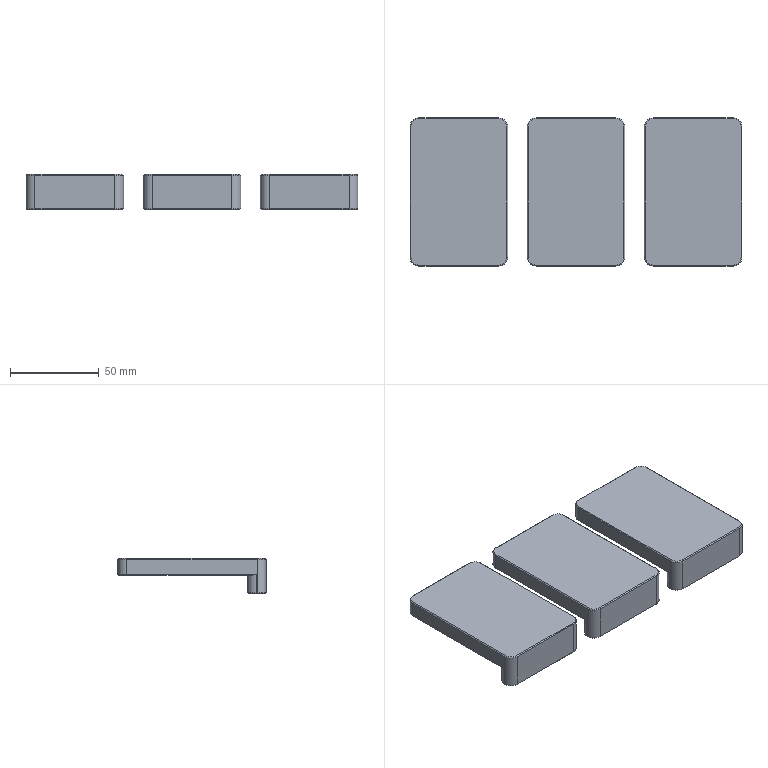NC program | NX | posted with a generic post | part box 187 x 83.5 x 20 mm
Whole program, first 1998 of 2119 lines:
N10 G17 G21 G94 G90
(FLOOR_WALL_COPY , TOOL : D80)
N12 T19 M6
N14 G54
N16 G17 G0 G90 X138.5 Y-41.747 S6500 M3
N18 G43 Z30. H19
N20 Z7.
N22 G94 G1 Z4. F1500.
N24 X133.5
N26 X-133.5
N28 Y-29.806
N30 Y9.75
N32 X133.5
N34 X138.5
N36 Z7.
N38 G0 Z30.
N40 Y-41.747
N42 Z6.
N44 G1 Z3.
N46 X133.5
N48 X-133.5
N50 Y-29.806
N52 Y9.75
N54 X133.5
N56 X138.5
N58 Z6.
N60 G0 Z30.
N62 Y-41.747
N64 Z5.
N66 G1 Z2.
N68 X133.5
N70 X-133.5
N72 Y9.75
N74 X133.5
N76 X138.5
N78 Z5.
N80 G0 Z30.
N82 Y-41.747
N84 Z4.
N86 G1 Z1.
N88 X133.5
N90 X-133.5
N92 Y9.75
N94 X133.5
N96 X138.5
N98 Z4.
N100 G0 Z30.
N102 Y-41.747
N104 Z3.
N106 G1 Z0.
N108 X133.5
N110 X-133.5
N112 Y9.75
N114 X133.5
N116 X138.5
N118 Z3.
N120 G0 Z30.
N122 M5
(FLOOR_WALL_1 , TOOL : D10)
N124 T15 M6
N126 G54
N128 G17 G0 G90 X-35.376 Y-46.25 S9500 M3
N130 G43 Z30. H15
N132 Z-7.4
N134 G94 G1 Z-10.4 F2500.
N136 X-43.489
N138 X-88.511
N140 G2 X-91.539 Y-45.751 R9.5
N142 G1 X-40.461
N144 G3 X-39.26 Y-45.251 R9.5
N146 G1 X-92.74
N148 G2 X-93.62 Y-44.752 R9.5
N150 G1 X-38.38
N152 G3 X-37.672 Y-44.253 R9.5
N154 G1 X-94.328
N156 G2 X-94.919 Y-43.753 R9.5
N158 G1 X-37.081
N160 G3 X-36.576 Y-43.254 R9.5
N162 G1 X-95.424
N164 G2 X-95.862 Y-42.755 R9.5
N166 G1 X-36.138
N168 G3 X-35.758 Y-42.255 R9.5
N170 G1 X-96.242
N172 G2 X-96.574 Y-41.756 R9.5
N174 G1 X-35.426
N176 G3 X-35.137 Y-41.257 R9.5
N178 G1 X-96.863
N180 G2 X-97.113 Y-40.757 R9.5
N182 G1 X-34.887
N184 G3 X-34.671 Y-40.258 R9.5
N186 G1 X-97.329
N188 G2 X-97.511 Y-39.759 R9.5
N190 G1 X-34.489
N192 G3 X-34.337 Y-39.259 R9.5
N194 G1 X-97.663
N196 G2 X-97.785 Y-38.76 R9.5
N198 G1 X-34.215
N200 G3 X-34.121 Y-38.261 R9.5
N202 G1 X-97.879
N204 G2 X-97.946 Y-37.761 R9.5
N206 G1 X-34.054
N208 G3 X-34.014 Y-37.262 R9.5
N210 G1 X-97.986
N212 G2 X-98. Y-36.763 R9.5
N214 G1 X-34.
N216 Y-36.75
N218 Y-36.263
N220 X-98.
N222 Y-35.764
N224 X-34.
N226 Y-35.265
N228 X-98.
N230 Y-34.765
N232 X-34.
N234 Y-34.266
N236 X-98.
N238 Y-33.767
N240 X-34.
N242 Y-33.267
N244 X-98.
N246 Y-32.768
N248 X-34.
N250 Y-32.269
N252 X-98.
N254 Y-31.769
N256 X-34.
N258 Y-31.27
N260 X-98.
N262 Y-30.771
N264 X-34.
N266 Y-30.271
N268 X-98.
N270 Y-29.772
N272 X-34.
N274 Y-29.273
N276 X-98.
N278 Y-28.773
N280 X-34.
N282 Y-28.274
N284 X-98.
N286 Y-27.775
N288 X-34.
N290 Y-27.275
N292 X-98.
N294 Y-26.776
N296 X-34.
N298 Y-26.277
N300 X-98.
N302 Y-25.777
N304 X-34.
N306 Y-25.278
N308 X-98.
N310 Y-24.779
N312 X-34.
N314 Y-24.279
N316 X-98.
N318 Y-23.78
N320 X-34.
N322 Y-23.281
N324 X-98.
N326 Y-22.781
N328 X-34.
N330 Y-22.282
N332 X-98.
N334 Y-21.783
N336 X-34.
N338 Y-21.283
N340 X-98.
N342 Y-20.784
N344 X-34.
N346 Y-20.285
N348 X-98.
N350 Y-19.785
N352 X-34.
N354 Y-19.286
N356 X-98.
N358 Y-18.787
N360 X-34.
N362 Y-18.287
N364 X-98.
N366 Y-17.788
N368 X-34.
N370 Y-17.289
N372 X-98.
N374 Y-16.789
N376 X-34.
N378 Y-16.29
N380 X-98.
N382 Y-15.791
N384 X-34.
N386 Y-15.291
N388 X-98.
N390 Y-14.792
N392 X-34.
N394 Y-14.293
N396 X-98.
N398 Y-13.793
N400 X-34.
N402 Y-13.294
N404 X-98.
N406 Y-12.795
N408 X-34.
N410 Y-12.295
N412 X-98.
N414 Y-11.796
N416 X-34.
N418 Y-11.297
N420 X-98.
N422 Y-10.797
N424 X-34.
N426 Y-10.298
N428 X-98.
N430 Y-9.799
N432 X-34.
N434 Y-9.299
N436 X-98.
N438 Y-8.8
N440 X-34.
N442 Y-8.301
N444 X-98.
N446 Y-7.801
N448 X-34.
N450 Y-7.302
N452 X-98.
N454 Y-6.803
N456 X-34.
N458 Y-6.303
N460 X-98.
N462 Y-5.804
N464 X-34.
N466 Y-5.305
N468 X-98.
N470 Y-4.805
N472 X-34.
N474 Y-4.306
N476 X-98.
N478 Y-3.807
N480 X-34.
N482 Y-3.307
N484 X-98.
N486 Y-2.808
N488 X-34.
N490 Y-2.309
N492 X-98.
N494 Y-1.809
N496 X-34.
N498 Y-1.31
N500 X-98.
N502 Y-0.811
N504 X-34.
N506 Y-0.311
N508 X-98.
N510 Y0.188
N512 X-34.
N514 Y0.687
N516 X-98.
N518 Y1.187
N520 X-34.
N522 Y1.686
N524 X-98.
N526 Y2.185
N528 X-34.
N530 Y2.685
N532 X-98.
N534 Y3.184
N536 X-34.
N538 Y3.683
N540 X-98.
N542 Y4.183
N544 X-34.
N546 Y4.682
N548 X-98.
N550 Y5.181
N552 X-34.
N554 Y5.681
N556 X-98.
N558 Y6.18
N560 X-34.
N562 Y6.679
N564 X-98.
N566 Y7.179
N568 X-34.
N570 Y7.678
N572 X-98.
N574 Y8.177
N576 X-34.
N578 Y8.677
N580 X-98.
N582 Y9.176
N584 X-34.
N586 Y9.675
N588 X-98.
N590 Y10.175
N592 X-34.
N594 Y10.674
N596 X-98.
N598 Y11.173
N600 X-34.
N602 Y11.673
N604 X-98.
N606 Y12.172
N608 X-34.
N610 Y12.671
N612 X-98.
N614 Y13.171
N616 X-34.
N618 Y13.67
N620 X-98.
N622 Y14.169
N624 X-34.
N626 Y14.669
N628 X-98.
N630 Y15.168
N632 X-34.
N634 Y15.667
N636 X-98.
N638 Y16.167
N640 X-34.
N642 Y16.666
N644 X-98.
N646 Y17.165
N648 X-34.
N650 Y17.665
N652 X-98.
N654 Y18.164
N656 X-34.
N658 Y18.663
N660 X-98.
N662 Y19.163
N664 X-34.
N666 Y19.662
N668 X-98.
N670 Y20.161
N672 X-34.
N674 Y20.661
N676 X-98.
N678 Y21.16
N680 X-34.
N682 Y21.659
N684 X-98.
N686 Y22.159
N688 X-34.
N690 Y22.658
N692 X-98.
N694 Y23.157
N696 X-34.
N698 Y23.657
N700 X-98.
N702 Y24.156
N704 X-34.
N706 Y24.655
N708 X-98.
N710 Y25.155
N712 X-34.
N714 Y25.654
N716 X-98.
N718 Y26.153
N720 X-89.54
N722 G2 X-91.804 Y26.653 R10.15
N724 G1 X-98.
N726 Y27.152
N728 X-93.
N730 G2 X-93.893 Y27.651 R10.15
N732 G1 X-98.
N734 Y28.151
N736 X-94.618
N738 G2 X-95.228 Y28.65 R10.15
N740 G1 X-98.
N742 Y29.149
N744 X-95.753
N746 G2 X-96.21 Y29.649 R10.15
N748 G1 X-98.
N750 Y30.148
N752 X-96.611
N754 G2 X-96.964 Y30.647 R10.15
N756 G1 X-98.
N758 Y31.147
N760 X-97.274
N762 X-101.
N764 Z-7.4
N766 G0 Z30.
N768 X-89.54 Y26.153
N770 Z-7.4
N772 G1 Z-10.4
N774 G3 X-88.5 Y26.1 R10.15
N776 G1 X-43.5
N778 G3 X-42.46 Y26.153 R10.15
N780 G1 X-34.
N782 Y26.653
N784 X-40.196
N786 G3 X-39. Y27.152 R10.15
N788 G1 X-34.
N790 Y27.651
N792 X-38.107
N794 G3 X-37.382 Y28.151 R10.15
N796 G1 X-34.
N798 Y28.65
N800 X-36.772
N802 G3 X-36.247 Y29.149 R10.15
N804 G1 X-34.
N806 Y29.649
N808 X-35.79
N810 G3 X-35.389 Y30.148 R10.15
N812 G1 X-34.
N814 Y30.647
N816 X-35.036
N818 G3 X-34.726 Y31.147 R10.15
N820 G1 X-34.
N822 X-32.5
N824 X-31. Y26.216
N826 Z-7.4
N828 G0 Z30.
N830 X30.624 Y-46.25
N832 Z-7.4
N834 G1 Z-10.4
N836 X22.512
N838 X-22.512
N840 G2 X-25.539 Y-45.751 R9.5
N842 G1 X25.539
N844 G3 X26.74 Y-45.251 R9.5
N846 G1 X-26.74
N848 G2 X-27.62 Y-44.752 R9.5
N850 G1 X27.62
N852 G3 X28.328 Y-44.253 R9.5
N854 G1 X-28.328
N856 G2 X-28.919 Y-43.753 R9.5
N858 G1 X28.919
N860 G3 X29.424 Y-43.254 R9.5
N862 G1 X-29.424
N864 G2 X-29.862 Y-42.755 R9.5
N866 G1 X29.862
N868 G3 X30.242 Y-42.255 R9.5
N870 G1 X-30.242
N872 G2 X-30.574 Y-41.756 R9.5
N874 G1 X30.574
N876 G3 X30.863 Y-41.257 R9.5
N878 G1 X-30.863
N880 G2 X-31.113 Y-40.757 R9.5
N882 G1 X31.113
N884 G3 X31.329 Y-40.258 R9.5
N886 G1 X-31.329
N888 G2 X-31.511 Y-39.759 R9.5
N890 G1 X31.511
N892 G3 X31.663 Y-39.259 R9.5
N894 G1 X-31.663
N896 G2 X-31.785 Y-38.76 R9.5
N898 G1 X31.785
N900 G3 X31.879 Y-38.261 R9.5
N902 G1 X-31.879
N904 G2 X-31.946 Y-37.761 R9.5
N906 G1 X31.946
N908 G3 X31.986 Y-37.262 R9.5
N910 G1 X-31.986
N912 G2 X-32. Y-36.763 R9.5
N914 G1 X32.
N916 Y-36.75
N918 Y-36.263
N920 X-32.
N922 Y-35.764
N924 X32.
N926 Y-35.265
N928 X-32.
N930 Y-34.765
N932 X32.
N934 Y-34.266
N936 X-32.
N938 Y-33.767
N940 X32.
N942 Y-33.267
N944 X-32.
N946 Y-32.768
N948 X32.
N950 Y-32.269
N952 X-32.
N954 Y-31.769
N956 X32.
N958 Y-31.27
N960 X-32.
N962 Y-30.771
N964 X32.
N966 Y-30.271
N968 X-32.
N970 Y-29.772
N972 X32.
N974 Y-29.273
N976 X-32.
N978 Y-28.773
N980 X32.
N982 Y-28.274
N984 X-32.
N986 Y-27.775
N988 X32.
N990 Y-27.275
N992 X-32.
N994 Y-26.776
N996 X32.
N998 Y-26.277
N1000 X-32.
N1002 Y-25.777
N1004 X32.
N1006 Y-25.278
N1008 X-32.
N1010 Y-24.779
N1012 X32.
N1014 Y-24.279
N1016 X-32.
N1018 Y-23.78
N1020 X32.
N1022 Y-23.281
N1024 X-32.
N1026 Y-22.781
N1028 X32.
N1030 Y-22.282
N1032 X-32.
N1034 Y-21.783
N1036 X32.
N1038 Y-21.283
N1040 X-32.
N1042 Y-20.784
N1044 X32.
N1046 Y-20.285
N1048 X-32.
N1050 Y-19.785
N1052 X32.
N1054 Y-19.286
N1056 X-32.
N1058 Y-18.787
N1060 X32.
N1062 Y-18.287
N1064 X-32.
N1066 Y-17.788
N1068 X32.
N1070 Y-17.289
N1072 X-32.
N1074 Y-16.789
N1076 X32.
N1078 Y-16.29
N1080 X-32.
N1082 Y-15.791
N1084 X32.
N1086 Y-15.291
N1088 X-32.
N1090 Y-14.792
N1092 X32.
N1094 Y-14.293
N1096 X-32.
N1098 Y-13.793
N1100 X32.
N1102 Y-13.294
N1104 X-32.
N1106 Y-12.795
N1108 X32.
N1110 Y-12.295
N1112 X-32.
N1114 Y-11.796
N1116 X32.
N1118 Y-11.297
N1120 X-32.
N1122 Y-10.797
N1124 X32.
N1126 Y-10.298
N1128 X-32.
N1130 Y-9.799
N1132 X32.
N1134 Y-9.299
N1136 X-32.
N1138 Y-8.8
N1140 X32.
N1142 Y-8.301
N1144 X-32.
N1146 Y-7.801
N1148 X32.
N1150 Y-7.302
N1152 X-32.
N1154 Y-6.803
N1156 X32.
N1158 Y-6.303
N1160 X-32.
N1162 Y-5.804
N1164 X32.
N1166 Y-5.305
N1168 X-32.
N1170 Y-4.805
N1172 X32.
N1174 Y-4.306
N1176 X-32.
N1178 Y-3.807
N1180 X32.
N1182 Y-3.307
N1184 X-32.
N1186 Y-2.808
N1188 X32.
N1190 Y-2.309
N1192 X-32.
N1194 Y-1.809
N1196 X32.
N1198 Y-1.31
N1200 X-32.
N1202 Y-0.811
N1204 X32.
N1206 Y-0.311
N1208 X-32.
N1210 Y0.188
N1212 X32.
N1214 Y0.687
N1216 X-32.
N1218 Y1.187
N1220 X32.
N1222 Y1.686
N1224 X-32.
N1226 Y2.185
N1228 X32.
N1230 Y2.685
N1232 X-32.
N1234 Y3.184
N1236 X32.
N1238 Y3.683
N1240 X-32.
N1242 Y4.183
N1244 X32.
N1246 Y4.682
N1248 X-32.
N1250 Y5.181
N1252 X32.
N1254 Y5.681
N1256 X-32.
N1258 Y6.18
N1260 X32.
N1262 Y6.679
N1264 X-32.
N1266 Y7.179
N1268 X32.
N1270 Y7.678
N1272 X-32.
N1274 Y8.177
N1276 X32.
N1278 Y8.677
N1280 X-32.
N1282 Y9.176
N1284 X32.
N1286 Y9.675
N1288 X-32.
N1290 Y10.175
N1292 X32.
N1294 Y10.674
N1296 X-32.
N1298 Y11.173
N1300 X32.
N1302 Y11.673
N1304 X-32.
N1306 Y12.172
N1308 X32.
N1310 Y12.671
N1312 X-32.
N1314 Y13.171
N1316 X32.
N1318 Y13.67
N1320 X-32.
N1322 Y14.169
N1324 X32.
N1326 Y14.669
N1328 X-32.
N1330 Y15.168
N1332 X32.
N1334 Y15.667
N1336 X-32.
N1338 Y16.167
N1340 X32.
N1342 Y16.666
N1344 X-32.
N1346 Y17.165
N1348 X32.
N1350 Y17.665
N1352 X-32.
N1354 Y18.164
N1356 X32.
N1358 Y18.663
N1360 X-32.
N1362 Y19.163
N1364 X32.
N1366 Y19.662
N1368 X-32.
N1370 Y20.161
N1372 X32.
N1374 Y20.661
N1376 X-32.
N1378 Y21.16
N1380 X32.
N1382 Y21.659
N1384 X-32.
N1386 Y22.159
N1388 X32.
N1390 Y22.658
N1392 X-32.
N1394 Y23.157
N1396 X32.
N1398 Y23.657
N1400 X-32.
N1402 Y24.156
N1404 X32.
N1406 Y24.655
N1408 X-32.
N1410 Y25.155
N1412 X32.
N1414 Y25.654
N1416 X-32.
N1418 Y26.153
N1420 X-23.54
N1422 G2 X-25.804 Y26.653 R10.15
N1424 G1 X-32.
N1426 Y27.152
N1428 X-27.
N1430 G2 X-27.893 Y27.651 R10.15
N1432 G1 X-32.
N1434 Y28.151
N1436 X-28.618
N1438 G2 X-29.228 Y28.65 R10.15
N1440 G1 X-32.
N1442 Y29.149
N1444 X-29.753
N1446 G2 X-30.21 Y29.649 R10.15
N1448 G1 X-32.
N1450 Y30.148
N1452 X-30.611
N1454 G2 X-30.964 Y30.647 R10.15
N1456 G1 X-32.
N1458 Y31.147
N1460 X-31.274
N1462 X-35. Y26.216
N1464 Z-7.4
N1466 G0 Z30.
N1468 X-23.54 Y26.153
N1470 Z-7.4
N1472 G1 Z-10.4
N1474 G3 X-22.5 Y26.1 R10.15
N1476 G1 X22.5
N1478 G3 X23.54 Y26.153 R10.15
N1480 G1 X32.
N1482 Y26.653
N1484 X25.804
N1486 G3 X27. Y27.152 R10.15
N1488 G1 X32.
N1490 Y27.651
N1492 X27.893
N1494 G3 X28.618 Y28.151 R10.15
N1496 G1 X32.
N1498 Y28.65
N1500 X29.228
N1502 G3 X29.753 Y29.149 R10.15
N1504 G1 X32.
N1506 Y29.649
N1508 X30.21
N1510 G3 X30.611 Y30.148 R10.15
N1512 G1 X32.
N1514 Y30.647
N1516 X30.964
N1518 G3 X31.274 Y31.147 R10.15
N1520 G1 X32.
N1522 X33.5
N1524 X35. Y26.216
N1526 Z-7.4
N1528 G0 Z30.
N1530 X96.624 Y-46.25
N1532 Z-7.4
N1534 G1 Z-10.4
N1536 X88.511
N1538 X43.489
N1540 G2 X40.461 Y-45.751 R9.5
N1542 G1 X91.539
N1544 G3 X92.74 Y-45.251 R9.5
N1546 G1 X39.26
N1548 G2 X38.38 Y-44.752 R9.5
N1550 G1 X93.62
N1552 G3 X94.328 Y-44.253 R9.5
N1554 G1 X37.672
N1556 G2 X37.081 Y-43.753 R9.5
N1558 G1 X94.919
N1560 G3 X95.424 Y-43.254 R9.5
N1562 G1 X36.576
N1564 G2 X36.138 Y-42.755 R9.5
N1566 G1 X95.862
N1568 G3 X96.242 Y-42.255 R9.5
N1570 G1 X35.758
N1572 G2 X35.426 Y-41.756 R9.5
N1574 G1 X96.574
N1576 G3 X96.863 Y-41.257 R9.5
N1578 G1 X35.137
N1580 G2 X34.887 Y-40.757 R9.5
N1582 G1 X97.113
N1584 G3 X97.329 Y-40.258 R9.5
N1586 G1 X34.671
N1588 G2 X34.489 Y-39.759 R9.5
N1590 G1 X97.511
N1592 G3 X97.663 Y-39.259 R9.5
N1594 G1 X34.337
N1596 G2 X34.215 Y-38.76 R9.5
N1598 G1 X97.785
N1600 G3 X97.879 Y-38.261 R9.5
N1602 G1 X34.121
N1604 G2 X34.054 Y-37.761 R9.5
N1606 G1 X97.946
N1608 G3 X97.986 Y-37.262 R9.5
N1610 G1 X34.014
N1612 G2 X34. Y-36.763 R9.5
N1614 G1 X98.
N1616 Y-36.75
N1618 Y-36.263
N1620 X34.
N1622 Y-35.764
N1624 X98.
N1626 Y-35.265
N1628 X34.
N1630 Y-34.765
N1632 X98.
N1634 Y-34.266
N1636 X34.
N1638 Y-33.767
N1640 X98.
N1642 Y-33.267
N1644 X34.
N1646 Y-32.768
N1648 X98.
N1650 Y-32.269
N1652 X34.
N1654 Y-31.769
N1656 X98.
N1658 Y-31.27
N1660 X34.
N1662 Y-30.771
N1664 X98.
N1666 Y-30.271
N1668 X34.
N1670 Y-29.772
N1672 X98.
N1674 Y-29.273
N1676 X34.
N1678 Y-28.773
N1680 X98.
N1682 Y-28.274
N1684 X34.
N1686 Y-27.775
N1688 X98.
N1690 Y-27.275
N1692 X34.
N1694 Y-26.776
N1696 X98.
N1698 Y-26.277
N1700 X34.
N1702 Y-25.777
N1704 X98.
N1706 Y-25.278
N1708 X34.
N1710 Y-24.779
N1712 X98.
N1714 Y-24.279
N1716 X34.
N1718 Y-23.78
N1720 X98.
N1722 Y-23.281
N1724 X34.
N1726 Y-22.781
N1728 X98.
N1730 Y-22.282
N1732 X34.
N1734 Y-21.783
N1736 X98.
N1738 Y-21.283
N1740 X34.
N1742 Y-20.784
N1744 X98.
N1746 Y-20.285
N1748 X34.
N1750 Y-19.785
N1752 X98.
N1754 Y-19.286
N1756 X34.
N1758 Y-18.787
N1760 X98.
N1762 Y-18.287
N1764 X34.
N1766 Y-17.788
N1768 X98.
N1770 Y-17.289
N1772 X34.
N1774 Y-16.789
N1776 X98.
N1778 Y-16.29
N1780 X34.
N1782 Y-15.791
N1784 X98.
N1786 Y-15.291
N1788 X34.
N1790 Y-14.792
N1792 X98.
N1794 Y-14.293
N1796 X34.
N1798 Y-13.793
N1800 X98.
N1802 Y-13.294
N1804 X34.
N1806 Y-12.795
N1808 X98.
N1810 Y-12.295
N1812 X34.
N1814 Y-11.796
N1816 X98.
N1818 Y-11.297
N1820 X34.
N1822 Y-10.797
N1824 X98.
N1826 Y-10.298
N1828 X34.
N1830 Y-9.799
N1832 X98.
N1834 Y-9.299
N1836 X34.
N1838 Y-8.8
N1840 X98.
N1842 Y-8.301
N1844 X34.
N1846 Y-7.801
N1848 X98.
N1850 Y-7.302
N1852 X34.
N1854 Y-6.803
N1856 X98.
N1858 Y-6.303
N1860 X34.
N1862 Y-5.804
N1864 X98.
N1866 Y-5.305
N1868 X34.
N1870 Y-4.805
N1872 X98.
N1874 Y-4.306
N1876 X34.
N1878 Y-3.807
N1880 X98.
N1882 Y-3.307
N1884 X34.
N1886 Y-2.808
N1888 X98.
N1890 Y-2.309
N1892 X34.
N1894 Y-1.809
N1896 X98.
N1898 Y-1.31
N1900 X34.
N1902 Y-0.811
N1904 X98.
N1906 Y-0.311
N1908 X34.
N1910 Y0.188
N1912 X98.
N1914 Y0.687
N1916 X34.
N1918 Y1.187
N1920 X98.
N1922 Y1.686
N1924 X34.
N1926 Y2.185
N1928 X98.
N1930 Y2.685
N1932 X34.
N1934 Y3.184
N1936 X98.
N1938 Y3.683
N1940 X34.
N1942 Y4.183
N1944 X98.
N1946 Y4.682
N1948 X34.
N1950 Y5.181
N1952 X98.
N1954 Y5.681
N1956 X34.
N1958 Y6.18
N1960 X98.
N1962 Y6.679
N1964 X34.
N1966 Y7.179
N1968 X98.
N1970 Y7.678
N1972 X34.
N1974 Y8.177
N1976 X98.
N1978 Y8.677
N1980 X34.
N1982 Y9.176
N1984 X98.
N1986 Y9.675
N1988 X34.
N1990 Y10.175
N1992 X98.
N1994 Y10.674
N1996 X34.
N1998 Y11.173
N2000 X98.
N2002 Y11.673
N2004 X34.
N2006 Y12.172
N2008 X98.
N2010 Y12.671
N2012 X34.
N2014 Y13.171
N2016 X98.
N2018 Y13.67
N2020 X34.
N2022 Y14.169
N2024 X98.
N2026 Y14.669
N2028 X34.
N2030 Y15.168
N2032 X98.
N2034 Y15.667
N2036 X34.
N2038 Y16.167
N2040 X98.
N2042 Y16.666
N2044 X34.
N2046 Y17.165
N2048 X98.
N2050 Y17.665
N2052 X34.
N2054 Y18.164
N2056 X98.
N2058 Y18.663
N2060 X34.
N2062 Y19.163
N2064 X98.
N2066 Y19.662
N2068 X34.
N2070 Y20.161
N2072 X98.
N2074 Y20.661
N2076 X34.
N2078 Y21.16
N2080 X98.
N2082 Y21.659
N2084 X34.
N2086 Y22.159
N2088 X98.
N2090 Y22.658
N2092 X34.
N2094 Y23.157
N2096 X98.
N2098 Y23.657
N2100 X34.
N2102 Y24.156
N2104 X98.
N2106 Y24.655
N2108 X34.
N2110 Y25.155
N2112 X98.
N2114 Y25.654
N2116 X34.
N2118 Y26.153
N2120 X42.46
N2122 G2 X40.196 Y26.653 R10.15
N2124 G1 X34.
N2126 Y27.152
N2128 X39.
N2130 G2 X38.107 Y27.651 R10.15
N2132 G1 X34.
N2134 Y28.151
N2136 X37.382
N2138 G2 X36.772 Y28.65 R10.15
N2140 G1 X34.
N2142 Y29.149
N2144 X36.247
N2146 G2 X35.79 Y29.649 R10.15
N2148 G1 X34.
N2150 Y30.148
N2152 X35.389
N2154 G2 X35.036 Y30.647 R10.15
N2156 G1 X34.
N2158 Y31.147
N2160 X34.726
N2162 X31. Y26.216
N2164 Z-7.4
N2166 G0 Z30.
N2168 X42.46 Y26.153
N2170 Z-7.4
N2172 G1 Z-10.4
N2174 G3 X43.5 Y26.1 R10.15
N2176 G1 X88.5
N2178 G3 X89.54 Y26.153 R10.15
N2180 G1 X98.
N2182 Y26.653
N2184 X91.804
N2186 G3 X93. Y27.152 R10.15
N2188 G1 X98.
N2190 Y27.651
N2192 X93.893
N2194 G3 X94.618 Y28.151 R10.15
N2196 G1 X98.
N2198 Y28.65
N2200 X95.228
N2202 G3 X95.753 Y29.149 R10.15
N2204 G1 X98.
N2206 Y29.649
N2208 X96.21
N2210 G3 X96.611 Y30.148 R10.15
N2212 G1 X98.
N2214 Y30.647
N2216 X96.964
N2218 G3 X97.274 Y31.147 R10.15
N2220 G1 X98.
N2222 X101.
N2224 Z-7.4
N2226 G0 Z30.
N2228 M5
(FLOOR_WALL_2 , TOOL : D10JING)
N2230 T14 M6
N2232 G54
N2234 G17 G0 G90 X-31.837 Y-41.247 S9500 M3
N2236 G43 Z30. H14
N2238 Z-7.5
N2240 G94 G1 Z-10.5 F1500.
N2242 X-35.132
N2244 X-96.868
N2246 G2 X-98. Y-36.75 R9.5
N2248 G1 Y-36.389
N2250 X-34.
N2252 Y-31.531
N2254 X-98.
N2256 Y-26.673
N2258 X-34.
N2260 Y-21.816
N2262 X-98.
N2264 Y-16.958
N2266 X-34.
N2268 Y-12.1
N2270 X-98.
N2272 Y-7.242
N2274 X-34.
N2276 Y-2.384
N2278 X-98.
N2280 Y2.474
N2282 X-34.
N2284 Y7.332
N2286 X-98.
N2288 Y12.19
N2290 X-34.
N2292 Y17.047
N2294 X-98.
N2296 Y21.905
N2298 X-34.
N2300 Y26.763
N2302 X-39.
N2304 Z-7.5
N2306 G0 Z30.
N2308 X-101.
N2310 Z-7.5
N2312 G1 Z-10.5
N2314 X-93.
N2316 X-98.
N2318 X-101.
N2320 Z-7.5
N2322 G0 Z30.
N2324 X-33. Y44.415
N2326 Z-7.5
N2328 G1 Z-10.5
N2330 X-33.066 Y35.879
N2332 X-34.03 Y33.038
N2334 G2 X-43.5 Y26.25 R10.
N2336 G1 X-88.5
N2338 G2 X-97.97 Y33.038 R10.
N2340 G1 X-100.727 Y41.166
N2342 Z-7.5
N2344 G0 Z30.
N2346 X34.163 Y-41.247
N2348 Z-7.5
N2350 G1 Z-10.5
N2352 X30.868
N2354 X-30.868
N2356 G2 X-32. Y-36.75 R9.5
N2358 G1 Y-36.389
N2360 X32.
N2362 Y-31.531
N2364 X-32.
N2366 Y-26.673
N2368 X32.
N2370 Y-21.816
N2372 X-32.
N2374 Y-16.958
N2376 X32.
N2378 Y-12.1
N2380 X-32.
N2382 Y-7.242
N2384 X32.
N2386 Y-2.384
N2388 X-32.
N2390 Y2.474
N2392 X32.
N2394 Y7.332
N2396 X-32.
N2398 Y12.19
N2400 X32.
N2402 Y17.047
N2404 X-32.
N2406 Y21.905
N2408 X32.
N2410 Y26.763
N2412 X27.
N2414 Z-7.5
N2416 G0 Z30.
N2418 X-35. Y26.414
N2420 Z-7.5
N2422 G1 Z-10.5
N2424 X-27. Y26.763
N2426 X-32.
N2428 X-35.
N2430 Y26.414
N2432 Z-7.5
N2434 G0 Z30.
N2436 X33. Y44.415
N2438 Z-7.5
N2440 G1 Z-10.5
N2442 X32.934 Y35.879
N2444 X31.97 Y33.038
N2446 G2 X22.5 Y26.25 R10.
N2448 G1 X-22.5
N2450 G2 X-31.97 Y33.038 R10.
N2452 G1 X-32.934 Y35.879
N2454 X-33. Y44.415
N2456 Z-7.5
N2458 G0 Z30.
N2460 X100.163 Y-41.247
N2462 Z-7.5
N2464 G1 Z-10.5
N2466 X96.868
N2468 X35.132
N2470 G2 X34. Y-36.751 R9.5
N2472 G1 Y-36.389
N2474 X98.
N2476 Y-31.531
N2478 X34.
N2480 Y-26.673
N2482 X98.
N2484 Y-21.816
N2486 X34.
N2488 Y-16.958
N2490 X98.
N2492 Y-12.1
N2494 X34.
N2496 Y-7.242
N2498 X98.
N2500 Y-2.384
N2502 X34.
N2504 Y2.474
N2506 X98.
N2508 Y7.332
N2510 X34.
N2512 Y12.19
N2514 X98.
N2516 Y17.047
N2518 X34.
N2520 Y21.905
N2522 X98.
N2524 Y26.763
N2526 X93.
N2528 X101.
N2530 Z-7.5
N2532 G0 Z30.
N2534 X31. Y26.414
N2536 Z-7.5
N2538 G1 Z-10.5
N2540 X39. Y26.763
N2542 X34.
N2544 X31.
N2546 Y26.414
N2548 Z-7.5
N2550 G0 Z30.
N2552 X100.727 Y41.166
N2554 Z-7.5
N2556 G1 Z-10.5
N2558 X97.97 Y33.038
N2560 G2 X88.5 Y26.25 R10.
N2562 G1 X43.5
N2564 G2 X34.03 Y33.038 R10.
N2566 G1 X33.066 Y35.879
N2568 X33. Y44.415
N2570 Z-7.5
N2572 G0 Z30.
N2574 M5
(HOLE_MILLING , TOOL : D4)
N2576 T11 M6
N2578 G54
N2580 G17 G0 G90 X-88.5 Y36.75 S9500 M3
N2582 G43 Z30. H11
N2584 Z0.5
N2586 G94 G3 X-88. Y36.25 R0.5 F1250.
N2588 X-87.5 Y36.75 R0.5
N2590 X-87.5 Y36.75 Z0.1 I-1. J0.
N2592 X-87.5 Y36.75 Z-0.3 I-1. J0.
N2594 X-87.5 Y36.75 Z-0.7 I-1. J0.
N2596 X-87.5 Y36.75 Z-1.1 I-1. J0.
N2598 X-87.5 Y36.75 Z-1.5 I-1. J0.
N2600 X-87.5 Y36.75 Z-1.9 I-1. J0.
N2602 X-87.5 Y36.75 Z-2.3 I-1. J0.
N2604 X-87.5 Y36.75 Z-2.7 I-1. J0.
N2606 X-87.5 Y36.75 Z-3.1 I-1. J0.
N2608 X-87.5 Y36.75 Z-3.5 I-1. J0.
N2610 X-87.5 Y36.75 Z-3.9 I-1. J0.
N2612 X-87.5 Y36.75 Z-4.3 I-1. J0.
N2614 X-87.5 Y36.75 Z-4.7 I-1. J0.
N2616 X-87.5 Y36.75 Z-5.1 I-1. J0.
N2618 X-87.5 Y36.75 Z-5.5 I-1. J0.
N2620 X-87.5 Y36.75 Z-5.9 I-1. J0.
N2622 X-87.5 Y36.75 Z-6.3 I-1. J0.
N2624 X-87.5 Y36.75 Z-6.7 I-1. J0.
N2626 X-87.5 Y36.75 Z-7.1 I-1. J0.
N2628 X-87.5 Y36.75 Z-7.5 I-1. J0.
N2630 X-87.5 Y36.75 Z-7.9 I-1. J0.
N2632 X-87.5 Y36.75 Z-8.3 I-1. J0.
N2634 X-87.5 Y36.75 Z-8.7 I-1. J0.
N2636 X-87.5 Y36.75 Z-9.1 I-1. J0.
N2638 X-87.5 Y36.75 Z-9.5 I-1. J0.
N2640 X-87.5 Y36.75 Z-9.9 I-1. J0.
N2642 X-87.5 Y36.75 Z-10.3 I-1. J0.
N2644 X-87.5 Y36.75 Z-10.7 I-1. J0.
N2646 X-87.5 Y36.75 Z-11.1 I-1. J0.
N2648 X-87.5 Y36.75 Z-11.5 I-1. J0.
N2650 X-87.5 Y36.75 Z-11.9 I-1. J0.
N2652 X-88.5 Y37.75 Z-12. R1.
N2654 X-89.5 Y36.75 R1.
N2656 X-88.5 Y37.75 R-1.
N2658 X-89. Y37.25 R0.5
N2660 X-88.5 Y36.75 R0.5
N2662 G0 Z30.
N2664 X-43.5
N2666 Z0.5
N2668 G3 X-43. Y36.25 R0.5
N2670 X-42.5 Y36.75 R0.5
N2672 X-42.5 Y36.75 Z0.1 I-1. J0.
N2674 X-42.5 Y36.75 Z-0.3 I-1. J0.
N2676 X-42.5 Y36.75 Z-0.7 I-1. J0.
N2678 X-42.5 Y36.75 Z-1.1 I-1. J0.
N2680 X-42.5 Y36.75 Z-1.5 I-1. J0.
N2682 X-42.5 Y36.75 Z-1.9 I-1. J0.
N2684 X-42.5 Y36.75 Z-2.3 I-1. J0.
N2686 X-42.5 Y36.75 Z-2.7 I-1. J0.
N2688 X-42.5 Y36.75 Z-3.1 I-1. J0.
N2690 X-42.5 Y36.75 Z-3.5 I-1. J0.
N2692 X-42.5 Y36.75 Z-3.9 I-1. J0.
N2694 X-42.5 Y36.75 Z-4.3 I-1. J0.
N2696 X-42.5 Y36.75 Z-4.7 I-1. J0.
N2698 X-42.5 Y36.75 Z-5.1 I-1. J0.
N2700 X-42.5 Y36.75 Z-5.5 I-1. J0.
N2702 X-42.5 Y36.75 Z-5.9 I-1. J0.
N2704 X-42.5 Y36.75 Z-6.3 I-1. J0.
N2706 X-42.5 Y36.75 Z-6.7 I-1. J0.
N2708 X-42.5 Y36.75 Z-7.1 I-1. J0.
N2710 X-42.5 Y36.75 Z-7.5 I-1. J0.
N2712 X-42.5 Y36.75 Z-7.9 I-1. J0.
N2714 X-42.5 Y36.75 Z-8.3 I-1. J0.
N2716 X-42.5 Y36.75 Z-8.7 I-1. J0.
N2718 X-42.5 Y36.75 Z-9.1 I-1. J0.
N2720 X-42.5 Y36.75 Z-9.5 I-1. J0.
N2722 X-42.5 Y36.75 Z-9.9 I-1. J0.
N2724 X-42.5 Y36.75 Z-10.3 I-1. J0.
N2726 X-42.5 Y36.75 Z-10.7 I-1. J0.
N2728 X-42.5 Y36.75 Z-11.1 I-1. J0.
N2730 X-42.5 Y36.75 Z-11.5 I-1. J0.
N2732 X-42.5 Y36.75 Z-11.9 I-1. J0.
N2734 X-43.5 Y37.75 Z-12. R1.
N2736 X-44.5 Y36.75 R1.
N2738 X-43.5 Y37.75 R-1.
N2740 X-44. Y37.25 R0.5
N2742 X-43.5 Y36.75 R0.5
N2744 G0 Z30.
N2746 X-22.5
N2748 Z0.5
N2750 G3 X-22. Y36.25 R0.5
N2752 X-21.5 Y36.75 R0.5
N2754 X-21.5 Y36.75 Z0.1 I-1. J0.
N2756 X-21.5 Y36.75 Z-0.3 I-1. J0.
N2758 X-21.5 Y36.75 Z-0.7 I-1. J0.
N2760 X-21.5 Y36.75 Z-1.1 I-1. J0.
N2762 X-21.5 Y36.75 Z-1.5 I-1. J0.
N2764 X-21.5 Y36.75 Z-1.9 I-1. J0.
N2766 X-21.5 Y36.75 Z-2.3 I-1. J0.
N2768 X-21.5 Y36.75 Z-2.7 I-1. J0.
N2770 X-21.5 Y36.75 Z-3.1 I-1. J0.
N2772 X-21.5 Y36.75 Z-3.5 I-1. J0.
N2774 X-21.5 Y36.75 Z-3.9 I-1. J0.
N2776 X-21.5 Y36.75 Z-4.3 I-1. J0.
N2778 X-21.5 Y36.75 Z-4.7 I-1. J0.
N2780 X-21.5 Y36.75 Z-5.1 I-1. J0.
N2782 X-21.5 Y36.75 Z-5.5 I-1. J0.
N2784 X-21.5 Y36.75 Z-5.9 I-1. J0.
N2786 X-21.5 Y36.75 Z-6.3 I-1. J0.
N2788 X-21.5 Y36.75 Z-6.7 I-1. J0.
N2790 X-21.5 Y36.75 Z-7.1 I-1. J0.
N2792 X-21.5 Y36.75 Z-7.5 I-1. J0.
N2794 X-21.5 Y36.75 Z-7.9 I-1. J0.
N2796 X-21.5 Y36.75 Z-8.3 I-1. J0.
N2798 X-21.5 Y36.75 Z-8.7 I-1. J0.
N2800 X-21.5 Y36.75 Z-9.1 I-1. J0.
N2802 X-21.5 Y36.75 Z-9.5 I-1. J0.
N2804 X-21.5 Y36.75 Z-9.9 I-1. J0.
N2806 X-21.5 Y36.75 Z-10.3 I-1. J0.
N2808 X-21.5 Y36.75 Z-10.7 I-1. J0.
N2810 X-21.5 Y36.75 Z-11.1 I-1. J0.
N2812 X-21.5 Y36.75 Z-11.5 I-1. J0.
N2814 X-21.5 Y36.75 Z-11.9 I-1. J0.
N2816 X-22.5 Y37.75 Z-12. R1.
N2818 X-23.5 Y36.75 R1.
N2820 X-22.5 Y37.75 R-1.
N2822 X-23. Y37.25 R0.5
N2824 X-22.5 Y36.75 R0.5
N2826 G0 Z30.
N2828 X22.5
N2830 Z0.5
N2832 G3 X23. Y36.25 R0.5
N2834 X23.5 Y36.75 R0.5
N2836 X23.5 Y36.75 Z0.1 I-1. J0.
N2838 X23.5 Y36.75 Z-0.3 I-1. J0.
N2840 X23.5 Y36.75 Z-0.7 I-1. J0.
N2842 X23.5 Y36.75 Z-1.1 I-1. J0.
N2844 X23.5 Y36.75 Z-1.5 I-1. J0.
N2846 X23.5 Y36.75 Z-1.9 I-1. J0.
N2848 X23.5 Y36.75 Z-2.3 I-1. J0.
N2850 X23.5 Y36.75 Z-2.7 I-1. J0.
N2852 X23.5 Y36.75 Z-3.1 I-1. J0.
N2854 X23.5 Y36.75 Z-3.5 I-1. J0.
N2856 X23.5 Y36.75 Z-3.9 I-1. J0.
N2858 X23.5 Y36.75 Z-4.3 I-1. J0.
N2860 X23.5 Y36.75 Z-4.7 I-1. J0.
N2862 X23.5 Y36.75 Z-5.1 I-1. J0.
N2864 X23.5 Y36.75 Z-5.5 I-1. J0.
N2866 X23.5 Y36.75 Z-5.9 I-1. J0.
N2868 X23.5 Y36.75 Z-6.3 I-1. J0.
N2870 X23.5 Y36.75 Z-6.7 I-1. J0.
N2872 X23.5 Y36.75 Z-7.1 I-1. J0.
N2874 X23.5 Y36.75 Z-7.5 I-1. J0.
N2876 X23.5 Y36.75 Z-7.9 I-1. J0.
N2878 X23.5 Y36.75 Z-8.3 I-1. J0.
N2880 X23.5 Y36.75 Z-8.7 I-1. J0.
N2882 X23.5 Y36.75 Z-9.1 I-1. J0.
N2884 X23.5 Y36.75 Z-9.5 I-1. J0.
N2886 X23.5 Y36.75 Z-9.9 I-1. J0.
N2888 X23.5 Y36.75 Z-10.3 I-1. J0.
N2890 X23.5 Y36.75 Z-10.7 I-1. J0.
N2892 X23.5 Y36.75 Z-11.1 I-1. J0.
N2894 X23.5 Y36.75 Z-11.5 I-1. J0.
N2896 X23.5 Y36.75 Z-11.9 I-1. J0.
N2898 X22.5 Y37.75 Z-12. R1.
N2900 X21.5 Y36.75 R1.
N2902 X22.5 Y37.75 R-1.
N2904 X22. Y37.25 R0.5
N2906 X22.5 Y36.75 R0.5
N2908 G0 Z30.
N2910 X43.5
N2912 Z0.5
N2914 G3 X44. Y36.25 R0.5
N2916 X44.5 Y36.75 R0.5
N2918 X44.5 Y36.75 Z0.1 I-1. J0.
N2920 X44.5 Y36.75 Z-0.3 I-1. J0.
N2922 X44.5 Y36.75 Z-0.7 I-1. J0.
N2924 X44.5 Y36.75 Z-1.1 I-1. J0.
N2926 X44.5 Y36.75 Z-1.5 I-1. J0.
N2928 X44.5 Y36.75 Z-1.9 I-1. J0.
N2930 X44.5 Y36.75 Z-2.3 I-1. J0.
N2932 X44.5 Y36.75 Z-2.7 I-1. J0.
N2934 X44.5 Y36.75 Z-3.1 I-1. J0.
N2936 X44.5 Y36.75 Z-3.5 I-1. J0.
N2938 X44.5 Y36.75 Z-3.9 I-1. J0.
N2940 X44.5 Y36.75 Z-4.3 I-1. J0.
N2942 X44.5 Y36.75 Z-4.7 I-1. J0.
N2944 X44.5 Y36.75 Z-5.1 I-1. J0.
N2946 X44.5 Y36.75 Z-5.5 I-1. J0.
N2948 X44.5 Y36.75 Z-5.9 I-1. J0.
N2950 X44.5 Y36.75 Z-6.3 I-1. J0.
N2952 X44.5 Y36.75 Z-6.7 I-1. J0.
N2954 X44.5 Y36.75 Z-7.1 I-1. J0.
N2956 X44.5 Y36.75 Z-7.5 I-1. J0.
N2958 X44.5 Y36.75 Z-7.9 I-1. J0.
N2960 X44.5 Y36.75 Z-8.3 I-1. J0.
N2962 X44.5 Y36.75 Z-8.7 I-1. J0.
N2964 X44.5 Y36.75 Z-9.1 I-1. J0.
N2966 X44.5 Y36.75 Z-9.5 I-1. J0.
N2968 X44.5 Y36.75 Z-9.9 I-1. J0.
N2970 X44.5 Y36.75 Z-10.3 I-1. J0.
N2972 X44.5 Y36.75 Z-10.7 I-1. J0.
N2974 X44.5 Y36.75 Z-11.1 I-1. J0.
N2976 X44.5 Y36.75 Z-11.5 I-1. J0.
N2978 X44.5 Y36.75 Z-11.9 I-1. J0.
N2980 X43.5 Y37.75 Z-12. R1.
N2982 X42.5 Y36.75 R1.
N2984 X43.5 Y37.75 R-1.
N2986 X43. Y37.25 R0.5
N2988 X43.5 Y36.75 R0.5
N2990 G0 Z30.
N2992 X88.5
N2994 Z0.5
N2996 G3 X89. Y36.25 R0.5
N2998 X89.5 Y36.75 R0.5
N3000 X89.5 Y36.75 Z0.1 I-1. J0.
N3002 X89.5 Y36.75 Z-0.3 I-1. J0.
N3004 X89.5 Y36.75 Z-0.7 I-1. J0.
N3006 X89.5 Y36.75 Z-1.1 I-1. J0.
N3008 X89.5 Y36.75 Z-1.5 I-1. J0.
N3010 X89.5 Y36.75 Z-1.9 I-1. J0.
N3012 X89.5 Y36.75 Z-2.3 I-1. J0.
N3014 X89.5 Y36.75 Z-2.7 I-1. J0.
N3016 X89.5 Y36.75 Z-3.1 I-1. J0.
N3018 X89.5 Y36.75 Z-3.5 I-1. J0.
N3020 X89.5 Y36.75 Z-3.9 I-1. J0.
N3022 X89.5 Y36.75 Z-4.3 I-1. J0.
N3024 X89.5 Y36.75 Z-4.7 I-1. J0.
N3026 X89.5 Y36.75 Z-5.1 I-1. J0.
N3028 X89.5 Y36.75 Z-5.5 I-1. J0.
N3030 X89.5 Y36.75 Z-5.9 I-1. J0.
N3032 X89.5 Y36.75 Z-6.3 I-1. J0.
N3034 X89.5 Y36.75 Z-6.7 I-1. J0.
N3036 X89.5 Y36.75 Z-7.1 I-1. J0.
N3038 X89.5 Y36.75 Z-7.5 I-1. J0.
N3040 X89.5 Y36.75 Z-7.9 I-1. J0.
N3042 X89.5 Y36.75 Z-8.3 I-1. J0.
N3044 X89.5 Y36.75 Z-8.7 I-1. J0.
N3046 X89.5 Y36.75 Z-9.1 I-1. J0.
N3048 X89.5 Y36.75 Z-9.5 I-1. J0.
N3050 X89.5 Y36.75 Z-9.9 I-1. J0.
N3052 X89.5 Y36.75 Z-10.3 I-1. J0.
N3054 X89.5 Y36.75 Z-10.7 I-1. J0.
N3056 X89.5 Y36.75 Z-11.1 I-1. J0.
N3058 X89.5 Y36.75 Z-11.5 I-1. J0.
N3060 X89.5 Y36.75 Z-11.9 I-1. J0.
N3062 X88.5 Y37.75 Z-12. R1.
N3064 X87.5 Y36.75 R1.
N3066 X88.5 Y37.75 R-1.
N3068 X88. Y37.25 R0.5
N3070 X88.5 Y36.75 R0.5
N3072 G0 Z30.
N3074 X73.5 Y-36.75
N3076 Z-10.
N3078 G3 X74. Y-37.25 R0.5
N3080 X74.5 Y-36.75 R0.5
N3082 X74.5 Y-36.75 Z-10.4 I-1. J0.
N3084 X74.5 Y-36.75 Z-10.8 I-1. J0.
N3086 X74.5 Y-36.75 Z-11.2 I-1. J0.
N3088 X74.5 Y-36.75 Z-11.6 I-1. J0.
N3090 X74.5 Y-36.75 Z-12. I-1. J0.
N3092 X74.5 Y-36.75 Z-12.4 I-1. J0.
N3094 X74.5 Y-36.75 Z-12.8 I-1. J0.
N3096 X74.5 Y-36.75 Z-13.2 I-1. J0.
N3098 X74.5 Y-36.75 Z-13.6 I-1. J0.
N3100 X74.5 Y-36.75 Z-14. I-1. J0.
N3102 X74.5 Y-36.75 Z-14.4 I-1. J0.
N3104 X74.5 Y-36.75 Z-14.8 I-1. J0.
N3106 X74.5 Y-36.75 Z-15.2 I-1. J0.
N3108 X74.5 Y-36.75 Z-15.6 I-1. J0.
N3110 X74.5 Y-36.75 Z-16. I-1. J0.
N3112 X74.5 Y-36.75 Z-16.4 I-1. J0.
N3114 X74.5 Y-36.75 Z-16.8 I-1. J0.
N3116 X74.5 Y-36.75 Z-17.2 I-1. J0.
N3118 X74.5 Y-36.75 Z-17.6 I-1. J0.
N3120 X74.5 Y-36.75 Z-18. I-1. J0.
N3122 X73.5 Y-35.75 R1.
N3124 X74.5 Y-36.75 R-1.
N3126 X74. Y-36.25 R0.5
N3128 X73.5 Y-36.75 R0.5
N3130 G0 Z30.
N3132 X58.5
N3134 Z-10.
N3136 G3 X59. Y-37.25 R0.5
N3138 X59.5 Y-36.75 R0.5
N3140 X59.5 Y-36.75 Z-10.4 I-1. J0.
N3142 X59.5 Y-36.75 Z-10.8 I-1. J0.
N3144 X59.5 Y-36.75 Z-11.2 I-1. J0.
N3146 X59.5 Y-36.75 Z-11.6 I-1. J0.
N3148 X59.5 Y-36.75 Z-12. I-1. J0.
N3150 X59.5 Y-36.75 Z-12.4 I-1. J0.
N3152 X59.5 Y-36.75 Z-12.8 I-1. J0.
N3154 X59.5 Y-36.75 Z-13.2 I-1. J0.
N3156 X59.5 Y-36.75 Z-13.6 I-1. J0.
N3158 X59.5 Y-36.75 Z-14. I-1. J0.
N3160 X59.5 Y-36.75 Z-14.4 I-1. J0.
N3162 X59.5 Y-36.75 Z-14.8 I-1. J0.
N3164 X59.5 Y-36.75 Z-15.2 I-1. J0.
N3166 X59.5 Y-36.75 Z-15.6 I-1. J0.
N3168 X59.5 Y-36.75 Z-16. I-1. J0.
N3170 X59.5 Y-36.75 Z-16.4 I-1. J0.
N3172 X59.5 Y-36.75 Z-16.8 I-1. J0.
N3174 X59.5 Y-36.75 Z-17.2 I-1. J0.
N3176 X59.5 Y-36.75 Z-17.6 I-1. J0.
N3178 X59.5 Y-36.75 Z-18. I-1. J0.
N3180 X58.5 Y-35.75 R1.
N3182 X59.5 Y-36.75 R-1.
N3184 X59. Y-36.25 R0.5
N3186 X58.5 Y-36.75 R0.5
N3188 G0 Z30.
N3190 X7.5
N3192 Z-10.
N3194 G3 X8. Y-37.25 R0.5
N3196 X8.5 Y-36.75 R0.5
N3198 X8.5 Y-36.75 Z-10.4 I-1. J0.
N3200 X8.5 Y-36.75 Z-10.8 I-1. J0.
N3202 X8.5 Y-36.75 Z-11.2 I-1. J0.
N3204 X8.5 Y-36.75 Z-11.6 I-1. J0.
N3206 X8.5 Y-36.75 Z-12. I-1. J0.
N3208 X8.5 Y-36.75 Z-12.4 I-1. J0.
N3210 X8.5 Y-36.75 Z-12.8 I-1. J0.
N3212 X8.5 Y-36.75 Z-13.2 I-1. J0.
N3214 X8.5 Y-36.75 Z-13.6 I-1. J0.
N3216 X8.5 Y-36.75 Z-14. I-1. J0.
N3218 X8.5 Y-36.75 Z-14.4 I-1. J0.
N3220 X8.5 Y-36.75 Z-14.8 I-1. J0.
N3222 X8.5 Y-36.75 Z-15.2 I-1. J0.
N3224 X8.5 Y-36.75 Z-15.6 I-1. J0.
N3226 X8.5 Y-36.75 Z-16. I-1. J0.
N3228 X8.5 Y-36.75 Z-16.4 I-1. J0.
N3230 X8.5 Y-36.75 Z-16.8 I-1. J0.
N3232 X8.5 Y-36.75 Z-17.2 I-1. J0.
N3234 X8.5 Y-36.75 Z-17.6 I-1. J0.
N3236 X8.5 Y-36.75 Z-18. I-1. J0.
N3238 X7.5 Y-35.75 R1.
N3240 X8.5 Y-36.75 R-1.
N3242 X8. Y-36.25 R0.5
N3244 X7.5 Y-36.75 R0.5
N3246 G0 Z30.
N3248 X-7.5
N3250 Z-10.
N3252 G3 X-7. Y-37.25 R0.5
N3254 X-6.5 Y-36.75 R0.5
N3256 X-6.5 Y-36.75 Z-10.4 I-1. J0.
N3258 X-6.5 Y-36.75 Z-10.8 I-1. J0.
N3260 X-6.5 Y-36.75 Z-11.2 I-1. J0.
N3262 X-6.5 Y-36.75 Z-11.6 I-1. J0.
N3264 X-6.5 Y-36.75 Z-12. I-1. J0.
N3266 X-6.5 Y-36.75 Z-12.4 I-1. J0.
N3268 X-6.5 Y-36.75 Z-12.8 I-1. J0.
N3270 X-6.5 Y-36.75 Z-13.2 I-1. J0.
N3272 X-6.5 Y-36.75 Z-13.6 I-1. J0.
N3274 X-6.5 Y-36.75 Z-14. I-1. J0.
N3276 X-6.5 Y-36.75 Z-14.4 I-1. J0.
N3278 X-6.5 Y-36.75 Z-14.8 I-1. J0.
N3280 X-6.5 Y-36.75 Z-15.2 I-1. J0.
N3282 X-6.5 Y-36.75 Z-15.6 I-1. J0.
N3284 X-6.5 Y-36.75 Z-16. I-1. J0.
N3286 X-6.5 Y-36.75 Z-16.4 I-1. J0.
N3288 X-6.5 Y-36.75 Z-16.8 I-1. J0.
N3290 X-6.5 Y-36.75 Z-17.2 I-1. J0.
N3292 X-6.5 Y-36.75 Z-17.6 I-1. J0.
N3294 X-6.5 Y-36.75 Z-18. I-1. J0.
N3296 X-7.5 Y-35.75 R1.
N3298 X-6.5 Y-36.75 R-1.
N3300 X-7. Y-36.25 R0.5
N3302 X-7.5 Y-36.75 R0.5
N3304 G0 Z30.
N3306 X-58.5
N3308 Z-10.
N3310 G3 X-58. Y-37.25 R0.5
N3312 X-57.5 Y-36.75 R0.5
N3314 X-57.5 Y-36.75 Z-10.4 I-1. J0.
N3316 X-57.5 Y-36.75 Z-10.8 I-1. J0.
N3318 X-57.5 Y-36.75 Z-11.2 I-1. J0.
N3320 X-57.5 Y-36.75 Z-11.6 I-1. J0.
N3322 X-57.5 Y-36.75 Z-12. I-1. J0.
N3324 X-57.5 Y-36.75 Z-12.4 I-1. J0.
N3326 X-57.5 Y-36.75 Z-12.8 I-1. J0.
N3328 X-57.5 Y-36.75 Z-13.2 I-1. J0.
N3330 X-57.5 Y-36.75 Z-13.6 I-1. J0.
N3332 X-57.5 Y-36.75 Z-14. I-1. J0.
N3334 X-57.5 Y-36.75 Z-14.4 I-1. J0.
N3336 X-57.5 Y-36.75 Z-14.8 I-1. J0.
N3338 X-57.5 Y-36.75 Z-15.2 I-1. J0.
N3340 X-57.5 Y-36.75 Z-15.6 I-1. J0.
N3342 X-57.5 Y-36.75 Z-16. I-1. J0.
N3344 X-57.5 Y-36.75 Z-16.4 I-1. J0.
N3346 X-57.5 Y-36.75 Z-16.8 I-1. J0.
N3348 X-57.5 Y-36.75 Z-17.2 I-1. J0.
N3350 X-57.5 Y-36.75 Z-17.6 I-1. J0.
N3352 X-57.5 Y-36.75 Z-18. I-1. J0.
N3354 X-58.5 Y-35.75 R1.
N3356 X-57.5 Y-36.75 R-1.
N3358 X-58. Y-36.25 R0.5
N3360 X-58.5 Y-36.75 R0.5
N3362 G0 Z30.
N3364 X-73.5
N3366 Z-10.
N3368 G3 X-73. Y-37.25 R0.5
N3370 X-72.5 Y-36.75 R0.5
N3372 X-72.5 Y-36.75 Z-10.4 I-1. J0.
N3374 X-72.5 Y-36.75 Z-10.8 I-1. J0.
N3376 X-72.5 Y-36.75 Z-11.2 I-1. J0.
N3378 X-72.5 Y-36.75 Z-11.6 I-1. J0.
N3380 X-72.5 Y-36.75 Z-12. I-1. J0.
N3382 X-72.5 Y-36.75 Z-12.4 I-1. J0.
N3384 X-72.5 Y-36.75 Z-12.8 I-1. J0.
N3386 X-72.5 Y-36.75 Z-13.2 I-1. J0.
N3388 X-72.5 Y-36.75 Z-13.6 I-1. J0.
N3390 X-72.5 Y-36.75 Z-14. I-1. J0.
N3392 X-72.5 Y-36.75 Z-14.4 I-1. J0.
N3394 X-72.5 Y-36.75 Z-14.8 I-1. J0.
N3396 X-72.5 Y-36.75 Z-15.2 I-1. J0.
N3398 X-72.5 Y-36.75 Z-15.6 I-1. J0.
N3400 X-72.5 Y-36.75 Z-16. I-1. J0.
N3402 X-72.5 Y-36.75 Z-16.4 I-1. J0.
N3404 X-72.5 Y-36.75 Z-16.8 I-1. J0.
N3406 X-72.5 Y-36.75 Z-17.2 I-1. J0.
N3408 X-72.5 Y-36.75 Z-17.6 I-1. J0.
N3410 X-72.5 Y-36.75 Z-18. I-1. J0.
N3412 X-73.5 Y-35.75 R1.
N3414 X-72.5 Y-36.75 R-1.
N3416 X-73. Y-36.25 R0.5
N3418 X-73.5 Y-36.75 R0.5
N3420 G0 Z30.
N3422 M5
(PLANAR_MILL_COPY_COPY_COPY_COPY_COPY , TOOL : D6A45)
N3424 T01 M6
N3426 G54
N3428 G17 G0 G90 X90.5 Y35.884 S9500 M3
N3430 G43 Z30. H1
N3432 Z0.
N3434 G94 G1 Z-1.5 F1250.
N3436 G3 X91. Y36.75 R1.
N3438 X88.5 Y39.25 R2.5
N3440 X91. Y36.75 R-2.5
N3442 X90.5 Y37.616 R1.
N3444 G1 Z0.
N3446 G0 Z30.
N3448 X66.866 Y29.75
N3450 Z0.
N3452 G1 Z-1.5
N3454 G3 X66. Y30.25 R1.
N3456 G1 X43.5
N3458 G2 X37.5 Y36.25 R6.
N3460 G1 Y36.75
N3462 G2 X43.5 Y42.75 R6.
N3464 G1 X88.5
N3466 G2 X94.5 Y36.75 R6.
N3468 G1 Y36.25
N3470 G2 X88.5 Y30.25 R6.
N3472 G1 X66.
N3474 G3 X65.134 Y29.75 R1.
N3476 G1 Z0.
N3478 G0 Z30.
N3480 X44.366 Y38.75
N3482 Z0.
N3484 G1 Z-1.5
N3486 G3 X43.5 Y39.25 R1.
N3488 X41. Y36.75 R2.5
N3490 X43.5 Y39.25 R-2.5
N3492 X42.634 Y38.75 R1.
N3494 G1 Z0.
N3496 G0 Z30.
N3498 X23.366
N3500 Z0.
N3502 G1 Z-1.5
N3504 G3 X22.5 Y39.25 R1.
N3506 X20. Y36.75 R2.5
N3508 X22.5 Y39.25 R-2.5
N3510 X21.634 Y38.75 R1.
N3512 G1 Z0.
N3514 G0 Z30.
N3516 X0.866 Y29.75
N3518 Z0.
N3520 G1 Z-1.5
N3522 G3 X0. Y30.25 R1.
N3524 G1 X-22.5
N3526 G2 X-28.5 Y36.25 R6.
N3528 G1 Y36.75
N3530 G2 X-22.5 Y42.75 R6.
N3532 G1 X22.5
N3534 G2 X28.5 Y36.75 R6.
N3536 G1 Y36.25
N3538 G2 X22.5 Y30.25 R6.
N3540 G1 X0.
N3542 G3 X-0.866 Y29.75 R1.
N3544 G1 Z0.
N3546 G0 Z30.
N3548 X-21.634 Y38.75
N3550 Z0.
N3552 G1 Z-1.5
N3554 G3 X-22.5 Y39.25 R1.
N3556 X-25. Y36.75 R2.5
N3558 X-22.5 Y39.25 R-2.5
N3560 X-23.366 Y38.75 R1.
N3562 G1 Z0.
N3564 G0 Z30.
N3566 X-42.634
N3568 Z0.
N3570 G1 Z-1.5
N3572 G3 X-43.5 Y39.25 R1.
N3574 X-46. Y36.75 R2.5
N3576 X-43.5 Y39.25 R-2.5
N3578 X-44.366 Y38.75 R1.
N3580 G1 Z0.
N3582 G0 Z30.
N3584 X-66.866 Y43.25
N3586 Z0.
N3588 G1 Z-1.5
N3590 G3 X-66. Y42.75 R1.
N3592 G1 X-43.5
N3594 G2 X-37.5 Y36.75 R6.
N3596 G1 Y36.25
N3598 G2 X-43.5 Y30.25 R6.
N3600 G1 X-88.5
N3602 G2 X-94.5 Y36.25 R6.
N3604 G1 Y36.75
N3606 G2 X-88.5 Y42.75 R6.
N3608 G1 X-66.
N3610 G3 X-65.134 Y43.25 R1.
N3612 G1 Z0.
N3614 G0 Z30.
N3616 X-87.634 Y38.75
N3618 Z0.
N3620 G1 Z-1.5
N3622 G3 X-88.5 Y39.25 R1.
N3624 X-91. Y36.75 R2.5
N3626 X-88.5 Y39.25 R-2.5
N3628 X-89.366 Y38.75 R1.
N3630 G1 Z0.
N3632 G0 Z30.
(PLANAR_MILL_COPY_COPY_COPY_COPY_COPY_COPY , TOOL : D6A45)
N3634 X-74.017 Y-37.943
N3636 Z-10.5
N3638 G1 Z-12.
N3640 X-74.366 Y-38.75
N3642 G3 X-73.5 Y-39.25 R1.
N3644 X-71. Y-36.75 R2.5
N3646 X-73.5 Y-39.25 R-2.5
N3648 X-72.634 Y-38.75 R1.
N3650 G1 X-72.983 Y-37.943
N3652 Z-10.5
N3654 G0 Z30.
N3656 X-59.017
N3658 Z-10.5
N3660 G1 Z-12.
N3662 X-59.366 Y-38.75
N3664 G3 X-58.5 Y-39.25 R1.
N3666 X-56. Y-36.75 R2.5
N3668 X-58.5 Y-39.25 R-2.5
N3670 X-57.634 Y-38.75 R1.
N3672 G1 X-57.983 Y-37.943
N3674 Z-10.5
N3676 G0 Z30.
N3678 X-8.017
N3680 Z-10.5
N3682 G1 Z-12.
N3684 X-8.366 Y-38.75
N3686 G3 X-7.5 Y-39.25 R1.
N3688 X-5. Y-36.75 R2.5
N3690 X-7.5 Y-39.25 R-2.5
N3692 X-6.634 Y-38.75 R1.
N3694 G1 X-6.983 Y-37.943
N3696 Z-10.5
N3698 G0 Z30.
N3700 X-35.84 Y30.299
N3702 Z-10.5
N3704 G1 Z-12.
N3706 X-36.534 Y30.486
N3708 G3 X-37.5 Y30.229 R1.
N3710 G1 Y-36.75
N3712 G2 X-43.5 Y-42.75 R6.
N3714 G1 X-88.5
N3716 G2 X-94.5 Y-36.75 R6.
N3718 G1 Y30.229
N3720 G3 X-95.466 Y30.486 R1.
N3722 G1 X-96.16 Y30.299
N3724 Z-10.5
N3726 G0 Z30.
N3728 X30.16
N3730 Z-10.5
N3732 G1 Z-12.
N3734 X29.466 Y30.486
N3736 G3 X28.5 Y30.229 R1.
N3738 G1 Y-36.75
N3740 G2 X22.5 Y-42.75 R6.
N3742 G1 X-22.5
N3744 G2 X-28.5 Y-36.75 R6.
N3746 G1 Y30.229
N3748 G3 X-29.466 Y30.486 R1.
N3750 G1 X-30.16 Y30.299
N3752 Z-10.5
N3754 G0 Z30.
N3756 X96.16
N3758 Z-10.5
N3760 G1 Z-12.
N3762 X95.466 Y30.486
N3764 G3 X94.5 Y30.229 R1.
N3766 G1 Y-36.75
N3768 G2 X88.5 Y-42.75 R6.
N3770 G1 X43.5
N3772 G2 X37.5 Y-36.75 R6.
N3774 G1 Y30.229
N3776 G3 X36.534 Y30.486 R1.
N3778 G1 X35.84 Y30.299
N3780 Z-10.5
N3782 G0 Z30.
N3784 X6.983 Y-37.943
N3786 Z-10.5
N3788 G1 Z-12.
N3790 X6.634 Y-38.75
N3792 G3 X7.5 Y-39.25 R1.
N3794 X10. Y-36.75 R2.5
N3796 X7.5 Y-39.25 R-2.5
N3798 X8.366 Y-38.75 R1.
N3800 G1 X8.017 Y-37.943
N3802 Z-10.5
N3804 G0 Z30.
N3806 X57.983
N3808 Z-10.5
N3810 G1 Z-12.
N3812 X57.634 Y-38.75
N3814 G3 X58.5 Y-39.25 R1.
N3816 X61. Y-36.75 R2.5
N3818 X58.5 Y-39.25 R-2.5
N3820 X59.366 Y-38.75 R1.
N3822 G1 X59.017 Y-37.943
N3824 Z-10.5
N3826 G0 Z30.
N3828 X72.983
N3830 Z-10.5
N3832 G1 Z-12.
N3834 X72.634 Y-38.75
N3836 G3 X73.5 Y-39.25 R1.
N3838 X76. Y-36.75 R2.5
N3840 X73.5 Y-39.25 R-2.5
N3842 X74.366 Y-38.75 R1.
N3844 G1 X74.017 Y-37.943
N3846 Z-10.5
N3848 G0 Z30.
N3850 M5
(HOLE_MILLING_COPY , TOOL : D4)
N3852 T11 M6
N3854 G54
N3856 G17 G0 G90 X-88.5 Y36.75 S9500 M3
N3858 G43 Z30. H11
N3860 Z0.5
N3862 G41 G94 G1 X-88.497 Y36.65 F1250. D11
N3864 G3 X-87.5 Y36.75 R0.504
N3866 X-87.5 Y36.75 Z-1.5 I-1. J0.
N3868 X-87.5 Y36.75 Z-3.5 I-1. J0.
N3870 X-87.5 Y36.75 Z-5.5 I-1. J0.
N3872 X-87.5 Y36.75 Z-7.5 I-1. J0.
N3874 X-87.5 Y36.75 Z-9.5 I-1. J0.
N3876 X-87.5 Y36.75 Z-11.5 I-1. J0.
N3878 X-88.5 Y37.75 Z-12. R1.
N3880 X-89.5 Y36.75 R1.
N3882 X-88.5 Y37.75 R-1.
N3884 X-88.6 Y36.753 R0.504
N3886 G40
N3888 G1 X-88.5 Y36.75
N3890 G0 Z30.
N3892 X-43.5
N3894 Z0.5
N3896 G41 G1 X-43.497 Y36.65
N3898 G3 X-42.5 Y36.75 R0.504
N3900 X-42.5 Y36.75 Z-1.5 I-1. J0.
N3902 X-42.5 Y36.75 Z-3.5 I-1. J0.
N3904 X-42.5 Y36.75 Z-5.5 I-1. J0.
N3906 X-42.5 Y36.75 Z-7.5 I-1. J0.
N3908 X-42.5 Y36.75 Z-9.5 I-1. J0.
N3910 X-42.5 Y36.75 Z-11.5 I-1. J0.
N3912 X-43.5 Y37.75 Z-12. R1.
N3914 X-44.5 Y36.75 R1.
N3916 X-43.5 Y37.75 R-1.
N3918 X-43.6 Y36.753 R0.504
N3920 G40
N3922 G1 X-43.5 Y36.75
N3924 G0 Z30.
N3926 X-22.5
N3928 Z0.5
N3930 G41 G1 X-22.497 Y36.65
N3932 G3 X-21.5 Y36.75 R0.504
N3934 X-21.5 Y36.75 Z-1.5 I-1. J0.
N3936 X-21.5 Y36.75 Z-3.5 I-1. J0.
N3938 X-21.5 Y36.75 Z-5.5 I-1. J0.
N3940 X-21.5 Y36.75 Z-7.5 I-1. J0.
N3942 X-21.5 Y36.75 Z-9.5 I-1. J0.
N3944 X-21.5 Y36.75 Z-11.5 I-1. J0.
N3946 X-22.5 Y37.75 Z-12. R1.
N3948 X-23.5 Y36.75 R1.
N3950 X-22.5 Y37.75 R-1.
N3952 X-22.6 Y36.753 R0.504
N3954 G40
N3956 G1 X-22.5 Y36.75
N3958 G0 Z30.
N3960 X22.5
N3962 Z0.5
N3964 G41 G1 X22.503 Y36.65
N3966 G3 X23.5 Y36.75 R0.504
N3968 X23.5 Y36.75 Z-1.5 I-1. J0.
N3970 X23.5 Y36.75 Z-3.5 I-1. J0.
N3972 X23.5 Y36.75 Z-5.5 I-1. J0.
N3974 X23.5 Y36.75 Z-7.5 I-1. J0.
N3976 X23.5 Y36.75 Z-9.5 I-1. J0.
N3978 X23.5 Y36.75 Z-11.5 I-1. J0.
N3980 X22.5 Y37.75 Z-12. R1.
N3982 X21.5 Y36.75 R1.
N3984 X22.5 Y37.75 R-1.
N3986 X22.4 Y36.753 R0.504
N3988 G40
N3990 G1 X22.5 Y36.75